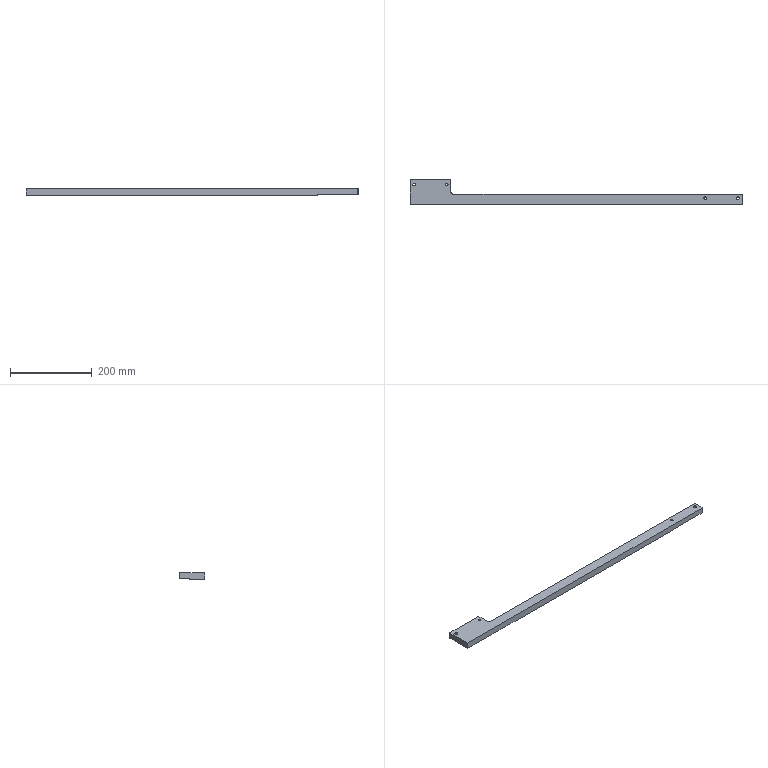Part | NX | features BREP 1 | 1 solid | 26 faces | box 812 x 62 x 16 mm | volume 388249 mm3 | plane 17 | cylinder 9 | commonest cylinder face diameters 6.5 x8 10 x1
STEP:
#1=CARTESIAN_POINT('',(798.75,16.,1.));
#2=VERTEX_POINT('',#1);
#3=CARTESIAN_POINT('',(805.25,16.,1.));
#4=VERTEX_POINT('',#3);
#5=CARTESIAN_POINT('',(802.,16.,1.));
#6=DIRECTION('',(0.,0.,1.));
#7=DIRECTION('',(1.,0.,0.));
#8=AXIS2_PLACEMENT_3D('',#5,#6,#7);
#9=CIRCLE('',#8,3.25);
#10=EDGE_CURVE('',#2,#4,#9,.T.);
#11=ORIENTED_EDGE('',*,*,#10,.F.);
#12=CARTESIAN_POINT('',(798.75,16.,16.));
#13=VERTEX_POINT('',#12);
#14=CARTESIAN_POINT('',(798.75,16.,16.));
#15=DIRECTION('',(0.,0.,1.));
#16=VECTOR('',#15,1000.);
#17=LINE('',#14,#16);
#18=EDGE_CURVE('',#13,#2,#17,.F.);
#19=ORIENTED_EDGE('',*,*,#18,.F.);
#20=CARTESIAN_POINT('',(805.25,16.,16.));
#21=VERTEX_POINT('',#20);
#22=CARTESIAN_POINT('',(802.,16.,16.));
#23=DIRECTION('',(0.,0.,1.));
#24=DIRECTION('',(1.,0.,0.));
#25=AXIS2_PLACEMENT_3D('',#22,#23,#24);
#26=CIRCLE('',#25,3.25);
#27=EDGE_CURVE('',#13,#21,#26,.T.);
#28=ORIENTED_EDGE('',*,*,#27,.T.);
#29=CARTESIAN_POINT('',(805.25,16.,16.));
#30=DIRECTION('',(0.,0.,1.));
#31=VECTOR('',#30,1000.);
#32=LINE('',#29,#31);
#33=EDGE_CURVE('',#21,#4,#32,.F.);
#34=ORIENTED_EDGE('',*,*,#33,.T.);
#35=EDGE_LOOP('',(#11,#19,#28,#34));
#36=FACE_BOUND('',#35,.T.);
#37=CARTESIAN_POINT('',(802.,16.,16.));
#38=DIRECTION('',(0.,0.,1.));
#39=DIRECTION('',(1.,0.,0.));
#40=AXIS2_PLACEMENT_3D('',#37,#38,#39);
#41=CYLINDRICAL_SURFACE('',#40,3.25);
#42=ADVANCED_FACE('',(#36),#41,.F.);
#43=CARTESIAN_POINT('',(718.75,16.,1.));
#44=VERTEX_POINT('',#43);
#45=CARTESIAN_POINT('',(725.25,16.,1.));
#46=VERTEX_POINT('',#45);
#47=CARTESIAN_POINT('',(722.,16.,1.));
#48=DIRECTION('',(0.,0.,1.));
#49=DIRECTION('',(1.,0.,0.));
#50=AXIS2_PLACEMENT_3D('',#47,#48,#49);
#51=CIRCLE('',#50,3.25);
#52=EDGE_CURVE('',#44,#46,#51,.T.);
#53=ORIENTED_EDGE('',*,*,#52,.F.);
#54=CARTESIAN_POINT('',(718.75,16.,16.));
#55=VERTEX_POINT('',#54);
#56=CARTESIAN_POINT('',(718.75,16.,16.));
#57=DIRECTION('',(0.,0.,1.));
#58=VECTOR('',#57,1000.);
#59=LINE('',#56,#58);
#60=EDGE_CURVE('',#55,#44,#59,.F.);
#61=ORIENTED_EDGE('',*,*,#60,.F.);
#62=CARTESIAN_POINT('',(725.25,16.,16.));
#63=VERTEX_POINT('',#62);
#64=CARTESIAN_POINT('',(722.,16.,16.));
#65=DIRECTION('',(0.,0.,1.));
#66=DIRECTION('',(1.,0.,0.));
#67=AXIS2_PLACEMENT_3D('',#64,#65,#66);
#68=CIRCLE('',#67,3.25);
#69=EDGE_CURVE('',#55,#63,#68,.T.);
#70=ORIENTED_EDGE('',*,*,#69,.T.);
#71=CARTESIAN_POINT('',(725.25,16.,16.));
#72=DIRECTION('',(0.,0.,1.));
#73=VECTOR('',#72,1000.);
#74=LINE('',#71,#73);
#75=EDGE_CURVE('',#63,#46,#74,.F.);
#76=ORIENTED_EDGE('',*,*,#75,.T.);
#77=EDGE_LOOP('',(#53,#61,#70,#76));
#78=FACE_BOUND('',#77,.T.);
#79=CARTESIAN_POINT('',(722.,16.,16.));
#80=DIRECTION('',(0.,0.,1.));
#81=DIRECTION('',(1.,0.,0.));
#82=AXIS2_PLACEMENT_3D('',#79,#80,#81);
#83=CYLINDRICAL_SURFACE('',#82,3.25);
#84=ADVANCED_FACE('',(#78),#83,.F.);
#85=CARTESIAN_POINT('',(6.75,49.,1.));
#86=VERTEX_POINT('',#85);
#87=CARTESIAN_POINT('',(13.25,49.,1.));
#88=VERTEX_POINT('',#87);
#89=CARTESIAN_POINT('',(10.,49.,1.));
#90=DIRECTION('',(0.,0.,1.));
#91=DIRECTION('',(1.,0.,0.));
#92=AXIS2_PLACEMENT_3D('',#89,#90,#91);
#93=CIRCLE('',#92,3.25);
#94=EDGE_CURVE('',#86,#88,#93,.T.);
#95=ORIENTED_EDGE('',*,*,#94,.F.);
#96=CARTESIAN_POINT('',(6.75,49.,16.));
#97=VERTEX_POINT('',#96);
#98=CARTESIAN_POINT('',(6.75,49.,16.));
#99=DIRECTION('',(0.,0.,1.));
#100=VECTOR('',#99,1000.);
#101=LINE('',#98,#100);
#102=EDGE_CURVE('',#97,#86,#101,.F.);
#103=ORIENTED_EDGE('',*,*,#102,.F.);
#104=CARTESIAN_POINT('',(13.25,49.,16.));
#105=VERTEX_POINT('',#104);
#106=CARTESIAN_POINT('',(10.,49.,16.));
#107=DIRECTION('',(0.,0.,1.));
#108=DIRECTION('',(1.,0.,0.));
#109=AXIS2_PLACEMENT_3D('',#106,#107,#108);
#110=CIRCLE('',#109,3.25);
#111=EDGE_CURVE('',#97,#105,#110,.T.);
#112=ORIENTED_EDGE('',*,*,#111,.T.);
#113=CARTESIAN_POINT('',(13.25,49.,16.));
#114=DIRECTION('',(0.,0.,1.));
#115=VECTOR('',#114,1000.);
#116=LINE('',#113,#115);
#117=EDGE_CURVE('',#105,#88,#116,.F.);
#118=ORIENTED_EDGE('',*,*,#117,.T.);
#119=EDGE_LOOP('',(#95,#103,#112,#118));
#120=FACE_BOUND('',#119,.T.);
#121=CARTESIAN_POINT('',(10.,49.,16.));
#122=DIRECTION('',(0.,0.,1.));
#123=DIRECTION('',(1.,0.,0.));
#124=AXIS2_PLACEMENT_3D('',#121,#122,#123);
#125=CYLINDRICAL_SURFACE('',#124,3.25);
#126=ADVANCED_FACE('',(#120),#125,.F.);
#127=CARTESIAN_POINT('',(86.75,49.,1.));
#128=VERTEX_POINT('',#127);
#129=CARTESIAN_POINT('',(93.25,49.,1.));
#130=VERTEX_POINT('',#129);
#131=CARTESIAN_POINT('',(90.,49.,1.));
#132=DIRECTION('',(0.,0.,1.));
#133=DIRECTION('',(1.,0.,0.));
#134=AXIS2_PLACEMENT_3D('',#131,#132,#133);
#135=CIRCLE('',#134,3.25);
#136=EDGE_CURVE('',#128,#130,#135,.T.);
#137=ORIENTED_EDGE('',*,*,#136,.F.);
#138=CARTESIAN_POINT('',(86.75,49.,16.));
#139=VERTEX_POINT('',#138);
#140=CARTESIAN_POINT('',(86.75,49.,16.));
#141=DIRECTION('',(0.,0.,1.));
#142=VECTOR('',#141,1000.);
#143=LINE('',#140,#142);
#144=EDGE_CURVE('',#139,#128,#143,.F.);
#145=ORIENTED_EDGE('',*,*,#144,.F.);
#146=CARTESIAN_POINT('',(93.25,49.,16.));
#147=VERTEX_POINT('',#146);
#148=CARTESIAN_POINT('',(90.,49.,16.));
#149=DIRECTION('',(0.,0.,1.));
#150=DIRECTION('',(1.,0.,0.));
#151=AXIS2_PLACEMENT_3D('',#148,#149,#150);
#152=CIRCLE('',#151,3.25);
#153=EDGE_CURVE('',#139,#147,#152,.T.);
#154=ORIENTED_EDGE('',*,*,#153,.T.);
#155=CARTESIAN_POINT('',(93.25,49.,16.));
#156=DIRECTION('',(0.,0.,1.));
#157=VECTOR('',#156,1000.);
#158=LINE('',#155,#157);
#159=EDGE_CURVE('',#147,#130,#158,.F.);
#160=ORIENTED_EDGE('',*,*,#159,.T.);
#161=EDGE_LOOP('',(#137,#145,#154,#160));
#162=FACE_BOUND('',#161,.T.);
#163=CARTESIAN_POINT('',(90.,49.,16.));
#164=DIRECTION('',(0.,0.,1.));
#165=DIRECTION('',(1.,0.,0.));
#166=AXIS2_PLACEMENT_3D('',#163,#164,#165);
#167=CYLINDRICAL_SURFACE('',#166,3.25);
#168=ADVANCED_FACE('',(#162),#167,.F.);
#169=CARTESIAN_POINT('',(1.,62.,1.));
#170=VERTEX_POINT('',#169);
#171=CARTESIAN_POINT('',(99.,62.,1.));
#172=VERTEX_POINT('',#171);
#173=CARTESIAN_POINT('',(0.,62.,1.));
#174=DIRECTION('',(1.,0.,0.));
#175=VECTOR('',#174,1000.);
#176=LINE('',#173,#175);
#177=EDGE_CURVE('',#170,#172,#176,.T.);
#178=ORIENTED_EDGE('',*,*,#177,.F.);
#179=CARTESIAN_POINT('',(1.,62.,16.));
#180=VERTEX_POINT('',#179);
#181=CARTESIAN_POINT('',(1.,62.,16.));
#182=DIRECTION('',(0.,0.,1.));
#183=VECTOR('',#182,1000.);
#184=LINE('',#181,#183);
#185=EDGE_CURVE('',#170,#180,#184,.T.);
#186=ORIENTED_EDGE('',*,*,#185,.T.);
#187=CARTESIAN_POINT('',(99.,62.,16.));
#188=VERTEX_POINT('',#187);
#189=CARTESIAN_POINT('',(100.,62.,16.));
#190=DIRECTION('',(-1.,0.,0.));
#191=VECTOR('',#190,1000.);
#192=LINE('',#189,#191);
#193=EDGE_CURVE('',#188,#180,#192,.T.);
#194=ORIENTED_EDGE('',*,*,#193,.F.);
#195=CARTESIAN_POINT('',(99.,62.,16.));
#196=DIRECTION('',(0.,0.,-1.));
#197=VECTOR('',#196,1000.);
#198=LINE('',#195,#197);
#199=EDGE_CURVE('',#188,#172,#198,.T.);
#200=ORIENTED_EDGE('',*,*,#199,.T.);
#201=EDGE_LOOP('',(#178,#186,#194,#200));
#202=FACE_BOUND('',#201,.T.);
#203=CARTESIAN_POINT('',(100.,62.,16.));
#204=DIRECTION('',(0.,-1.,0.));
#205=DIRECTION('',(0.,0.,-1.));
#206=AXIS2_PLACEMENT_3D('',#203,#204,#205);
#207=PLANE('',#206);
#208=ADVANCED_FACE('',(#202),#207,.F.);
#209=CARTESIAN_POINT('',(100.,61.,1.));
#210=VERTEX_POINT('',#209);
#211=CARTESIAN_POINT('',(100.,61.,16.));
#212=VERTEX_POINT('',#211);
#213=CARTESIAN_POINT('',(100.,61.,16.));
#214=DIRECTION('',(0.,0.,1.));
#215=VECTOR('',#214,1000.);
#216=LINE('',#213,#215);
#217=EDGE_CURVE('',#210,#212,#216,.T.);
#218=ORIENTED_EDGE('',*,*,#217,.F.);
#219=CARTESIAN_POINT('',(99.,62.,1.));
#220=DIRECTION('',(-0.7071,0.7071,0.));
#221=VECTOR('',#220,1000.);
#222=LINE('',#219,#221);
#223=EDGE_CURVE('',#210,#172,#222,.T.);
#224=ORIENTED_EDGE('',*,*,#223,.T.);
#225=ORIENTED_EDGE('',*,*,#199,.F.);
#226=CARTESIAN_POINT('',(80.5,80.5,16.));
#227=DIRECTION('',(-0.7071,0.7071,0.));
#228=VECTOR('',#227,1000.);
#229=LINE('',#226,#228);
#230=EDGE_CURVE('',#212,#188,#229,.T.);
#231=ORIENTED_EDGE('',*,*,#230,.F.);
#232=EDGE_LOOP('',(#218,#224,#225,#231));
#233=FACE_BOUND('',#232,.T.);
#234=CARTESIAN_POINT('',(99.,62.,16.));
#235=DIRECTION('',(-0.7071,-0.7071,0.));
#236=DIRECTION('',(-0.7071,0.7071,0.));
#237=AXIS2_PLACEMENT_3D('',#234,#235,#236);
#238=PLANE('',#237);
#239=ADVANCED_FACE('',(#233),#238,.F.);
#240=ORIENTED_EDGE('',*,*,#185,.F.);
#241=CARTESIAN_POINT('',(0.,61.,1.));
#242=VERTEX_POINT('',#241);
#243=CARTESIAN_POINT('',(0.,61.,1.));
#244=DIRECTION('',(-0.7071,-0.7071,0.));
#245=VECTOR('',#244,1000.);
#246=LINE('',#243,#245);
#247=EDGE_CURVE('',#170,#242,#246,.T.);
#248=ORIENTED_EDGE('',*,*,#247,.T.);
#249=CARTESIAN_POINT('',(0.,61.,16.));
#250=VERTEX_POINT('',#249);
#251=CARTESIAN_POINT('',(0.,61.,16.));
#252=DIRECTION('',(0.,0.,-1.));
#253=VECTOR('',#252,1000.);
#254=LINE('',#251,#253);
#255=EDGE_CURVE('',#250,#242,#254,.T.);
#256=ORIENTED_EDGE('',*,*,#255,.F.);
#257=CARTESIAN_POINT('',(-30.5,30.5,16.));
#258=DIRECTION('',(-0.7071,-0.7071,0.));
#259=VECTOR('',#258,1000.);
#260=LINE('',#257,#259);
#261=EDGE_CURVE('',#180,#250,#260,.T.);
#262=ORIENTED_EDGE('',*,*,#261,.F.);
#263=EDGE_LOOP('',(#240,#248,#256,#262));
#264=FACE_BOUND('',#263,.T.);
#265=CARTESIAN_POINT('',(0.,61.,16.));
#266=DIRECTION('',(0.7071,-0.7071,0.));
#267=DIRECTION('',(0.,0.,-1.));
#268=AXIS2_PLACEMENT_3D('',#265,#266,#267);
#269=PLANE('',#268);
#270=ADVANCED_FACE('',(#264),#269,.F.);
#271=CARTESIAN_POINT('',(0.,36.,1.));
#272=VERTEX_POINT('',#271);
#273=CARTESIAN_POINT('',(0.,36.,1.));
#274=DIRECTION('',(0.,1.,0.));
#275=VECTOR('',#274,1000.);
#276=LINE('',#273,#275);
#277=EDGE_CURVE('',#272,#242,#276,.T.);
#278=ORIENTED_EDGE('',*,*,#277,.F.);
#279=CARTESIAN_POINT('',(0.,36.,0.));
#280=VERTEX_POINT('',#279);
#281=CARTESIAN_POINT('',(0.,36.,1.));
#282=DIRECTION('',(0.,0.,-1.));
#283=VECTOR('',#282,1000.);
#284=LINE('',#281,#283);
#285=EDGE_CURVE('',#272,#280,#284,.T.);
#286=ORIENTED_EDGE('',*,*,#285,.T.);
#287=CARTESIAN_POINT('',(0.,1.,0.));
#288=VERTEX_POINT('',#287);
#289=CARTESIAN_POINT('',(0.,62.,0.));
#290=DIRECTION('',(0.,-1.,0.));
#291=VECTOR('',#290,1000.);
#292=LINE('',#289,#291);
#293=EDGE_CURVE('',#280,#288,#292,.T.);
#294=ORIENTED_EDGE('',*,*,#293,.T.);
#295=CARTESIAN_POINT('',(0.,1.,16.));
#296=VERTEX_POINT('',#295);
#297=CARTESIAN_POINT('',(0.,1.,16.));
#298=DIRECTION('',(0.,0.,1.));
#299=VECTOR('',#298,1000.);
#300=LINE('',#297,#299);
#301=EDGE_CURVE('',#288,#296,#300,.T.);
#302=ORIENTED_EDGE('',*,*,#301,.T.);
#303=CARTESIAN_POINT('',(0.,62.,16.));
#304=DIRECTION('',(0.,-1.,0.));
#305=VECTOR('',#304,1000.);
#306=LINE('',#303,#305);
#307=EDGE_CURVE('',#250,#296,#306,.T.);
#308=ORIENTED_EDGE('',*,*,#307,.F.);
#309=ORIENTED_EDGE('',*,*,#255,.T.);
#310=EDGE_LOOP('',(#278,#286,#294,#302,#308,#309));
#311=FACE_BOUND('',#310,.T.);
#312=CARTESIAN_POINT('',(0.,62.,16.));
#313=DIRECTION('',(1.,0.,0.));
#314=DIRECTION('',(0.,1.,0.));
#315=AXIS2_PLACEMENT_3D('',#312,#313,#314);
#316=PLANE('',#315);
#317=ADVANCED_FACE('',(#311),#316,.F.);
#318=CARTESIAN_POINT('',(1.,0.,0.));
#319=VERTEX_POINT('',#318);
#320=CARTESIAN_POINT('',(712.,0.,0.));
#321=VERTEX_POINT('',#320);
#322=CARTESIAN_POINT('',(0.,0.,0.));
#323=DIRECTION('',(1.,0.,0.));
#324=VECTOR('',#323,1000.);
#325=LINE('',#322,#324);
#326=EDGE_CURVE('',#319,#321,#325,.T.);
#327=ORIENTED_EDGE('',*,*,#326,.T.);
#328=CARTESIAN_POINT('',(712.,0.,1.));
#329=VERTEX_POINT('',#328);
#330=CARTESIAN_POINT('',(712.,0.,16.));
#331=DIRECTION('',(0.,0.,1.));
#332=VECTOR('',#331,1000.);
#333=LINE('',#330,#332);
#334=EDGE_CURVE('',#321,#329,#333,.T.);
#335=ORIENTED_EDGE('',*,*,#334,.T.);
#336=CARTESIAN_POINT('',(811.,0.,1.));
#337=VERTEX_POINT('',#336);
#338=CARTESIAN_POINT('',(0.,0.,1.));
#339=DIRECTION('',(1.,0.,0.));
#340=VECTOR('',#339,1000.);
#341=LINE('',#338,#340);
#342=EDGE_CURVE('',#329,#337,#341,.T.);
#343=ORIENTED_EDGE('',*,*,#342,.T.);
#344=CARTESIAN_POINT('',(811.,0.,16.));
#345=VERTEX_POINT('',#344);
#346=CARTESIAN_POINT('',(811.,0.,16.));
#347=DIRECTION('',(0.,0.,1.));
#348=VECTOR('',#347,1000.);
#349=LINE('',#346,#348);
#350=EDGE_CURVE('',#337,#345,#349,.T.);
#351=ORIENTED_EDGE('',*,*,#350,.T.);
#352=CARTESIAN_POINT('',(1.,0.,16.));
#353=VERTEX_POINT('',#352);
#354=CARTESIAN_POINT('',(0.,0.,16.));
#355=DIRECTION('',(1.,0.,0.));
#356=VECTOR('',#355,1000.);
#357=LINE('',#354,#356);
#358=EDGE_CURVE('',#353,#345,#357,.T.);
#359=ORIENTED_EDGE('',*,*,#358,.F.);
#360=CARTESIAN_POINT('',(1.,0.,16.));
#361=DIRECTION('',(0.,0.,-1.));
#362=VECTOR('',#361,1000.);
#363=LINE('',#360,#362);
#364=EDGE_CURVE('',#353,#319,#363,.T.);
#365=ORIENTED_EDGE('',*,*,#364,.T.);
#366=EDGE_LOOP('',(#327,#335,#343,#351,#359,#365));
#367=FACE_BOUND('',#366,.T.);
#368=CARTESIAN_POINT('',(0.,0.,16.));
#369=DIRECTION('',(0.,1.,0.));
#370=DIRECTION('',(1.,0.,0.));
#371=AXIS2_PLACEMENT_3D('',#368,#369,#370);
#372=PLANE('',#371);
#373=ADVANCED_FACE('',(#367),#372,.F.);
#374=CARTESIAN_POINT('',(812.,1.,16.));
#375=VERTEX_POINT('',#374);
#376=CARTESIAN_POINT('',(812.,1.,1.));
#377=VERTEX_POINT('',#376);
#378=CARTESIAN_POINT('',(812.,1.,16.));
#379=DIRECTION('',(0.,0.,-1.));
#380=VECTOR('',#379,1000.);
#381=LINE('',#378,#380);
#382=EDGE_CURVE('',#375,#377,#381,.T.);
#383=ORIENTED_EDGE('',*,*,#382,.T.);
#384=CARTESIAN_POINT('',(812.,25.,1.));
#385=VERTEX_POINT('',#384);
#386=CARTESIAN_POINT('',(812.,26.,1.));
#387=DIRECTION('',(0.,-1.,0.));
#388=VECTOR('',#387,1000.);
#389=LINE('',#386,#388);
#390=EDGE_CURVE('',#385,#377,#389,.T.);
#391=ORIENTED_EDGE('',*,*,#390,.F.);
#392=CARTESIAN_POINT('',(812.,25.,16.));
#393=VERTEX_POINT('',#392);
#394=CARTESIAN_POINT('',(812.,25.,16.));
#395=DIRECTION('',(0.,0.,1.));
#396=VECTOR('',#395,1000.);
#397=LINE('',#394,#396);
#398=EDGE_CURVE('',#385,#393,#397,.T.);
#399=ORIENTED_EDGE('',*,*,#398,.T.);
#400=CARTESIAN_POINT('',(812.,0.,16.));
#401=DIRECTION('',(0.,1.,0.));
#402=VECTOR('',#401,1000.);
#403=LINE('',#400,#402);
#404=EDGE_CURVE('',#375,#393,#403,.T.);
#405=ORIENTED_EDGE('',*,*,#404,.F.);
#406=EDGE_LOOP('',(#383,#391,#399,#405));
#407=FACE_BOUND('',#406,.T.);
#408=CARTESIAN_POINT('',(812.,0.,16.));
#409=DIRECTION('',(-1.,0.,0.));
#410=DIRECTION('',(0.,0.,1.));
#411=AXIS2_PLACEMENT_3D('',#408,#409,#410);
#412=PLANE('',#411);
#413=ADVANCED_FACE('',(#407),#412,.F.);
#414=CARTESIAN_POINT('',(712.,26.,1.));
#415=VERTEX_POINT('',#414);
#416=CARTESIAN_POINT('',(811.,26.,1.));
#417=VERTEX_POINT('',#416);
#418=CARTESIAN_POINT('',(712.,26.,1.));
#419=DIRECTION('',(1.,0.,0.));
#420=VECTOR('',#419,1000.);
#421=LINE('',#418,#420);
#422=EDGE_CURVE('',#415,#417,#421,.T.);
#423=ORIENTED_EDGE('',*,*,#422,.F.);
#424=CARTESIAN_POINT('',(712.,26.,0.));
#425=VERTEX_POINT('',#424);
#426=CARTESIAN_POINT('',(712.,26.,1.));
#427=DIRECTION('',(0.,0.,-1.));
#428=VECTOR('',#427,1000.);
#429=LINE('',#426,#428);
#430=EDGE_CURVE('',#415,#425,#429,.T.);
#431=ORIENTED_EDGE('',*,*,#430,.T.);
#432=CARTESIAN_POINT('',(105.,26.,0.));
#433=VERTEX_POINT('',#432);
#434=CARTESIAN_POINT('',(812.,26.,0.));
#435=DIRECTION('',(-1.,0.,0.));
#436=VECTOR('',#435,1000.);
#437=LINE('',#434,#436);
#438=EDGE_CURVE('',#425,#433,#437,.T.);
#439=ORIENTED_EDGE('',*,*,#438,.T.);
#440=CARTESIAN_POINT('',(105.,26.,16.));
#441=VERTEX_POINT('',#440);
#442=CARTESIAN_POINT('',(105.,26.,16.));
#443=DIRECTION('',(0.,0.,1.));
#444=VECTOR('',#443,1000.);
#445=LINE('',#442,#444);
#446=EDGE_CURVE('',#433,#441,#445,.T.);
#447=ORIENTED_EDGE('',*,*,#446,.T.);
#448=CARTESIAN_POINT('',(811.,26.,16.));
#449=VERTEX_POINT('',#448);
#450=CARTESIAN_POINT('',(812.,26.,16.));
#451=DIRECTION('',(-1.,0.,0.));
#452=VECTOR('',#451,1000.);
#453=LINE('',#450,#452);
#454=EDGE_CURVE('',#449,#441,#453,.T.);
#455=ORIENTED_EDGE('',*,*,#454,.F.);
#456=CARTESIAN_POINT('',(811.,26.,16.));
#457=DIRECTION('',(0.,0.,-1.));
#458=VECTOR('',#457,1000.);
#459=LINE('',#456,#458);
#460=EDGE_CURVE('',#449,#417,#459,.T.);
#461=ORIENTED_EDGE('',*,*,#460,.T.);
#462=EDGE_LOOP('',(#423,#431,#439,#447,#455,#461));
#463=FACE_BOUND('',#462,.T.);
#464=CARTESIAN_POINT('',(812.,26.,16.));
#465=DIRECTION('',(0.,-1.,0.));
#466=DIRECTION('',(0.,0.,-1.));
#467=AXIS2_PLACEMENT_3D('',#464,#465,#466);
#468=PLANE('',#467);
#469=ADVANCED_FACE('',(#463),#468,.F.);
#470=CARTESIAN_POINT('',(100.,31.,0.));
#471=VERTEX_POINT('',#470);
#472=CARTESIAN_POINT('',(100.,36.,0.));
#473=VERTEX_POINT('',#472);
#474=CARTESIAN_POINT('',(100.,26.,0.));
#475=DIRECTION('',(0.,1.,0.));
#476=VECTOR('',#475,1000.);
#477=LINE('',#474,#476);
#478=EDGE_CURVE('',#471,#473,#477,.T.);
#479=ORIENTED_EDGE('',*,*,#478,.T.);
#480=CARTESIAN_POINT('',(100.,36.,1.));
#481=VERTEX_POINT('',#480);
#482=CARTESIAN_POINT('',(100.,36.,1.));
#483=DIRECTION('',(0.,0.,-1.));
#484=VECTOR('',#483,1000.);
#485=LINE('',#482,#484);
#486=EDGE_CURVE('',#481,#473,#485,.T.);
#487=ORIENTED_EDGE('',*,*,#486,.F.);
#488=CARTESIAN_POINT('',(100.,36.,1.));
#489=DIRECTION('',(0.,-1.,0.));
#490=VECTOR('',#489,1000.);
#491=LINE('',#488,#490);
#492=EDGE_CURVE('',#210,#481,#491,.T.);
#493=ORIENTED_EDGE('',*,*,#492,.F.);
#494=ORIENTED_EDGE('',*,*,#217,.T.);
#495=CARTESIAN_POINT('',(100.,31.,16.));
#496=VERTEX_POINT('',#495);
#497=CARTESIAN_POINT('',(100.,26.,16.));
#498=DIRECTION('',(0.,1.,0.));
#499=VECTOR('',#498,1000.);
#500=LINE('',#497,#499);
#501=EDGE_CURVE('',#496,#212,#500,.T.);
#502=ORIENTED_EDGE('',*,*,#501,.F.);
#503=CARTESIAN_POINT('',(100.,31.,0.));
#504=DIRECTION('',(0.,0.,-1.));
#505=VECTOR('',#504,1000.);
#506=LINE('',#503,#505);
#507=EDGE_CURVE('',#496,#471,#506,.T.);
#508=ORIENTED_EDGE('',*,*,#507,.T.);
#509=EDGE_LOOP('',(#479,#487,#493,#494,#502,#508));
#510=FACE_BOUND('',#509,.T.);
#511=CARTESIAN_POINT('',(100.,26.,16.));
#512=DIRECTION('',(-1.,0.,0.));
#513=DIRECTION('',(0.,0.,1.));
#514=AXIS2_PLACEMENT_3D('',#511,#512,#513);
#515=PLANE('',#514);
#516=ADVANCED_FACE('',(#510),#515,.F.);
#517=ORIENTED_EDGE('',*,*,#358,.T.);
#518=CARTESIAN_POINT('',(405.5,-405.5,16.));
#519=DIRECTION('',(0.7071,0.7071,0.));
#520=VECTOR('',#519,1000.);
#521=LINE('',#518,#520);
#522=EDGE_CURVE('',#345,#375,#521,.T.);
#523=ORIENTED_EDGE('',*,*,#522,.T.);
#524=ORIENTED_EDGE('',*,*,#404,.T.);
#525=CARTESIAN_POINT('',(418.5,418.5,16.));
#526=DIRECTION('',(-0.7071,0.7071,0.));
#527=VECTOR('',#526,1000.);
#528=LINE('',#525,#527);
#529=EDGE_CURVE('',#393,#449,#528,.T.);
#530=ORIENTED_EDGE('',*,*,#529,.T.);
#531=ORIENTED_EDGE('',*,*,#454,.T.);
#532=CARTESIAN_POINT('',(105.,31.,16.));
#533=DIRECTION('',(0.,0.,-1.));
#534=DIRECTION('',(1.,0.,0.));
#535=AXIS2_PLACEMENT_3D('',#532,#533,#534);
#536=CIRCLE('',#535,5.);
#537=EDGE_CURVE('',#441,#496,#536,.T.);
#538=ORIENTED_EDGE('',*,*,#537,.T.);
#539=ORIENTED_EDGE('',*,*,#501,.T.);
#540=ORIENTED_EDGE('',*,*,#230,.T.);
#541=ORIENTED_EDGE('',*,*,#193,.T.);
#542=ORIENTED_EDGE('',*,*,#261,.T.);
#543=ORIENTED_EDGE('',*,*,#307,.T.);
#544=CARTESIAN_POINT('',(0.5,0.5,16.));
#545=DIRECTION('',(0.7071,-0.7071,0.));
#546=VECTOR('',#545,1000.);
#547=LINE('',#544,#546);
#548=EDGE_CURVE('',#296,#353,#547,.T.);
#549=ORIENTED_EDGE('',*,*,#548,.T.);
#550=EDGE_LOOP('',(#517,#523,#524,#530,#531,#538,#539,#540,#541,#542,#543,#549));
#551=FACE_BOUND('',#550,.T.);
#552=CARTESIAN_POINT('',(802.,16.,16.));
#553=DIRECTION('',(0.,0.,1.));
#554=DIRECTION('',(1.,0.,0.));
#555=AXIS2_PLACEMENT_3D('',#552,#553,#554);
#556=CIRCLE('',#555,3.25);
#557=EDGE_CURVE('',#21,#13,#556,.T.);
#558=ORIENTED_EDGE('',*,*,#557,.F.);
#559=ORIENTED_EDGE('',*,*,#27,.F.);
#560=EDGE_LOOP('',(#558,#559));
#561=FACE_BOUND('',#560,.T.);
#562=CARTESIAN_POINT('',(722.,16.,16.));
#563=DIRECTION('',(0.,0.,1.));
#564=DIRECTION('',(1.,0.,0.));
#565=AXIS2_PLACEMENT_3D('',#562,#563,#564);
#566=CIRCLE('',#565,3.25);
#567=EDGE_CURVE('',#63,#55,#566,.T.);
#568=ORIENTED_EDGE('',*,*,#567,.F.);
#569=ORIENTED_EDGE('',*,*,#69,.F.);
#570=EDGE_LOOP('',(#568,#569));
#571=FACE_BOUND('',#570,.T.);
#572=CARTESIAN_POINT('',(10.,49.,16.));
#573=DIRECTION('',(0.,0.,1.));
#574=DIRECTION('',(1.,0.,0.));
#575=AXIS2_PLACEMENT_3D('',#572,#573,#574);
#576=CIRCLE('',#575,3.25);
#577=EDGE_CURVE('',#105,#97,#576,.T.);
#578=ORIENTED_EDGE('',*,*,#577,.F.);
#579=ORIENTED_EDGE('',*,*,#111,.F.);
#580=EDGE_LOOP('',(#578,#579));
#581=FACE_BOUND('',#580,.T.);
#582=CARTESIAN_POINT('',(90.,49.,16.));
#583=DIRECTION('',(0.,0.,1.));
#584=DIRECTION('',(1.,0.,0.));
#585=AXIS2_PLACEMENT_3D('',#582,#583,#584);
#586=CIRCLE('',#585,3.25);
#587=EDGE_CURVE('',#147,#139,#586,.T.);
#588=ORIENTED_EDGE('',*,*,#587,.F.);
#589=ORIENTED_EDGE('',*,*,#153,.F.);
#590=EDGE_LOOP('',(#588,#589));
#591=FACE_BOUND('',#590,.T.);
#592=CARTESIAN_POINT('',(0.,0.,16.));
#593=DIRECTION('',(0.,0.,1.));
#594=DIRECTION('',(1.,0.,0.));
#595=AXIS2_PLACEMENT_3D('',#592,#593,#594);
#596=PLANE('',#595);
#597=ADVANCED_FACE('',(#551,#561,#571,#581,#591),#596,.T.);
#598=ORIENTED_EDGE('',*,*,#438,.F.);
#599=CARTESIAN_POINT('',(712.,26.,0.));
#600=DIRECTION('',(0.,1.,0.));
#601=VECTOR('',#600,1000.);
#602=LINE('',#599,#601);
#603=EDGE_CURVE('',#321,#425,#602,.T.);
#604=ORIENTED_EDGE('',*,*,#603,.F.);
#605=ORIENTED_EDGE('',*,*,#326,.F.);
#606=CARTESIAN_POINT('',(1.,0.,0.));
#607=DIRECTION('',(-0.7071,0.7071,0.));
#608=VECTOR('',#607,1000.);
#609=LINE('',#606,#608);
#610=EDGE_CURVE('',#319,#288,#609,.T.);
#611=ORIENTED_EDGE('',*,*,#610,.T.);
#612=ORIENTED_EDGE('',*,*,#293,.F.);
#613=CARTESIAN_POINT('',(0.,36.,0.));
#614=DIRECTION('',(-1.,0.,0.));
#615=VECTOR('',#614,1000.);
#616=LINE('',#613,#615);
#617=EDGE_CURVE('',#473,#280,#616,.T.);
#618=ORIENTED_EDGE('',*,*,#617,.F.);
#619=ORIENTED_EDGE('',*,*,#478,.F.);
#620=CARTESIAN_POINT('',(105.,31.,0.));
#621=DIRECTION('',(0.,0.,1.));
#622=DIRECTION('',(1.,0.,0.));
#623=AXIS2_PLACEMENT_3D('',#620,#621,#622);
#624=CIRCLE('',#623,5.);
#625=EDGE_CURVE('',#471,#433,#624,.T.);
#626=ORIENTED_EDGE('',*,*,#625,.T.);
#627=EDGE_LOOP('',(#598,#604,#605,#611,#612,#618,#619,#626));
#628=FACE_BOUND('',#627,.T.);
#629=CARTESIAN_POINT('',(0.,0.,0.));
#630=DIRECTION('',(0.,0.,1.));
#631=DIRECTION('',(1.,0.,0.));
#632=AXIS2_PLACEMENT_3D('',#629,#630,#631);
#633=PLANE('',#632);
#634=ADVANCED_FACE('',(#628),#633,.F.);
#635=CARTESIAN_POINT('',(812.,1.,1.));
#636=DIRECTION('',(-0.7071,-0.7071,0.));
#637=VECTOR('',#636,1000.);
#638=LINE('',#635,#637);
#639=EDGE_CURVE('',#377,#337,#638,.T.);
#640=ORIENTED_EDGE('',*,*,#639,.F.);
#641=ORIENTED_EDGE('',*,*,#382,.F.);
#642=ORIENTED_EDGE('',*,*,#522,.F.);
#643=ORIENTED_EDGE('',*,*,#350,.F.);
#644=EDGE_LOOP('',(#640,#641,#642,#643));
#645=FACE_BOUND('',#644,.T.);
#646=CARTESIAN_POINT('',(812.,1.,16.));
#647=DIRECTION('',(-0.7071,0.7071,0.));
#648=DIRECTION('',(0.,0.,1.));
#649=AXIS2_PLACEMENT_3D('',#646,#647,#648);
#650=PLANE('',#649);
#651=ADVANCED_FACE('',(#645),#650,.F.);
#652=CARTESIAN_POINT('',(811.,26.,1.));
#653=DIRECTION('',(0.7071,-0.7071,0.));
#654=VECTOR('',#653,1000.);
#655=LINE('',#652,#654);
#656=EDGE_CURVE('',#417,#385,#655,.T.);
#657=ORIENTED_EDGE('',*,*,#656,.F.);
#658=ORIENTED_EDGE('',*,*,#460,.F.);
#659=ORIENTED_EDGE('',*,*,#529,.F.);
#660=ORIENTED_EDGE('',*,*,#398,.F.);
#661=EDGE_LOOP('',(#657,#658,#659,#660));
#662=FACE_BOUND('',#661,.T.);
#663=CARTESIAN_POINT('',(811.,26.,16.));
#664=DIRECTION('',(-0.7071,-0.7071,0.));
#665=DIRECTION('',(-0.7071,0.7071,0.));
#666=AXIS2_PLACEMENT_3D('',#663,#664,#665);
#667=PLANE('',#666);
#668=ADVANCED_FACE('',(#662),#667,.F.);
#669=ORIENTED_EDGE('',*,*,#548,.F.);
#670=ORIENTED_EDGE('',*,*,#301,.F.);
#671=ORIENTED_EDGE('',*,*,#610,.F.);
#672=ORIENTED_EDGE('',*,*,#364,.F.);
#673=EDGE_LOOP('',(#669,#670,#671,#672));
#674=FACE_BOUND('',#673,.T.);
#675=CARTESIAN_POINT('',(1.,0.,16.));
#676=DIRECTION('',(0.7071,0.7071,0.));
#677=DIRECTION('',(0.,0.,-1.));
#678=AXIS2_PLACEMENT_3D('',#675,#676,#677);
#679=PLANE('',#678);
#680=ADVANCED_FACE('',(#674),#679,.F.);
#681=ORIENTED_EDGE('',*,*,#537,.F.);
#682=ORIENTED_EDGE('',*,*,#446,.F.);
#683=ORIENTED_EDGE('',*,*,#625,.F.);
#684=ORIENTED_EDGE('',*,*,#507,.F.);
#685=EDGE_LOOP('',(#681,#682,#683,#684));
#686=FACE_BOUND('',#685,.T.);
#687=CARTESIAN_POINT('',(105.,31.,16.));
#688=DIRECTION('',(0.,0.,1.));
#689=DIRECTION('',(1.,0.,0.));
#690=AXIS2_PLACEMENT_3D('',#687,#688,#689);
#691=CYLINDRICAL_SURFACE('',#690,5.);
#692=ADVANCED_FACE('',(#686),#691,.F.);
#693=ORIENTED_EDGE('',*,*,#617,.T.);
#694=ORIENTED_EDGE('',*,*,#285,.F.);
#695=CARTESIAN_POINT('',(0.,36.,1.));
#696=DIRECTION('',(-1.,0.,0.));
#697=VECTOR('',#696,1000.);
#698=LINE('',#695,#697);
#699=EDGE_CURVE('',#481,#272,#698,.T.);
#700=ORIENTED_EDGE('',*,*,#699,.F.);
#701=ORIENTED_EDGE('',*,*,#486,.T.);
#702=EDGE_LOOP('',(#693,#694,#700,#701));
#703=FACE_BOUND('',#702,.T.);
#704=CARTESIAN_POINT('',(0.,36.,1.));
#705=DIRECTION('',(0.,-1.,0.));
#706=DIRECTION('',(-1.,0.,0.));
#707=AXIS2_PLACEMENT_3D('',#704,#705,#706);
#708=PLANE('',#707);
#709=ADVANCED_FACE('',(#703),#708,.F.);
#710=ORIENTED_EDGE('',*,*,#492,.T.);
#711=ORIENTED_EDGE('',*,*,#699,.T.);
#712=ORIENTED_EDGE('',*,*,#277,.T.);
#713=ORIENTED_EDGE('',*,*,#247,.F.);
#714=ORIENTED_EDGE('',*,*,#177,.T.);
#715=ORIENTED_EDGE('',*,*,#223,.F.);
#716=EDGE_LOOP('',(#710,#711,#712,#713,#714,#715));
#717=FACE_BOUND('',#716,.T.);
#718=CARTESIAN_POINT('',(10.,49.,1.));
#719=DIRECTION('',(0.,0.,1.));
#720=DIRECTION('',(1.,0.,0.));
#721=AXIS2_PLACEMENT_3D('',#718,#719,#720);
#722=CIRCLE('',#721,3.25);
#723=EDGE_CURVE('',#88,#86,#722,.T.);
#724=ORIENTED_EDGE('',*,*,#723,.T.);
#725=ORIENTED_EDGE('',*,*,#94,.T.);
#726=EDGE_LOOP('',(#724,#725));
#727=FACE_BOUND('',#726,.T.);
#728=CARTESIAN_POINT('',(90.,49.,1.));
#729=DIRECTION('',(0.,0.,1.));
#730=DIRECTION('',(1.,0.,0.));
#731=AXIS2_PLACEMENT_3D('',#728,#729,#730);
#732=CIRCLE('',#731,3.25);
#733=EDGE_CURVE('',#130,#128,#732,.T.);
#734=ORIENTED_EDGE('',*,*,#733,.T.);
#735=ORIENTED_EDGE('',*,*,#136,.T.);
#736=EDGE_LOOP('',(#734,#735));
#737=FACE_BOUND('',#736,.T.);
#738=CARTESIAN_POINT('',(0.,0.,1.));
#739=DIRECTION('',(0.,0.,-1.));
#740=DIRECTION('',(0.,-1.,0.));
#741=AXIS2_PLACEMENT_3D('',#738,#739,#740);
#742=PLANE('',#741);
#743=ADVANCED_FACE('',(#717,#727,#737),#742,.T.);
#744=ORIENTED_EDGE('',*,*,#603,.T.);
#745=ORIENTED_EDGE('',*,*,#430,.F.);
#746=CARTESIAN_POINT('',(712.,26.,1.));
#747=DIRECTION('',(0.,1.,0.));
#748=VECTOR('',#747,1000.);
#749=LINE('',#746,#748);
#750=EDGE_CURVE('',#329,#415,#749,.T.);
#751=ORIENTED_EDGE('',*,*,#750,.F.);
#752=ORIENTED_EDGE('',*,*,#334,.F.);
#753=EDGE_LOOP('',(#744,#745,#751,#752));
#754=FACE_BOUND('',#753,.T.);
#755=CARTESIAN_POINT('',(712.,26.,1.));
#756=DIRECTION('',(-1.,0.,0.));
#757=DIRECTION('',(0.,0.,1.));
#758=AXIS2_PLACEMENT_3D('',#755,#756,#757);
#759=PLANE('',#758);
#760=ADVANCED_FACE('',(#754),#759,.F.);
#761=ORIENTED_EDGE('',*,*,#750,.T.);
#762=ORIENTED_EDGE('',*,*,#422,.T.);
#763=ORIENTED_EDGE('',*,*,#656,.T.);
#764=ORIENTED_EDGE('',*,*,#390,.T.);
#765=ORIENTED_EDGE('',*,*,#639,.T.);
#766=ORIENTED_EDGE('',*,*,#342,.F.);
#767=EDGE_LOOP('',(#761,#762,#763,#764,#765,#766));
#768=FACE_BOUND('',#767,.T.);
#769=CARTESIAN_POINT('',(802.,16.,1.));
#770=DIRECTION('',(0.,0.,1.));
#771=DIRECTION('',(1.,0.,0.));
#772=AXIS2_PLACEMENT_3D('',#769,#770,#771);
#773=CIRCLE('',#772,3.25);
#774=EDGE_CURVE('',#4,#2,#773,.T.);
#775=ORIENTED_EDGE('',*,*,#774,.T.);
#776=ORIENTED_EDGE('',*,*,#10,.T.);
#777=EDGE_LOOP('',(#775,#776));
#778=FACE_BOUND('',#777,.T.);
#779=CARTESIAN_POINT('',(722.,16.,1.));
#780=DIRECTION('',(0.,0.,1.));
#781=DIRECTION('',(1.,0.,0.));
#782=AXIS2_PLACEMENT_3D('',#779,#780,#781);
#783=CIRCLE('',#782,3.25);
#784=EDGE_CURVE('',#46,#44,#783,.T.);
#785=ORIENTED_EDGE('',*,*,#784,.T.);
#786=ORIENTED_EDGE('',*,*,#52,.T.);
#787=EDGE_LOOP('',(#785,#786));
#788=FACE_BOUND('',#787,.T.);
#789=CARTESIAN_POINT('',(0.,0.,1.));
#790=DIRECTION('',(0.,0.,1.));
#791=DIRECTION('',(1.,0.,0.));
#792=AXIS2_PLACEMENT_3D('',#789,#790,#791);
#793=PLANE('',#792);
#794=ADVANCED_FACE('',(#768,#778,#788),#793,.F.);
#795=ORIENTED_EDGE('',*,*,#144,.T.);
#796=ORIENTED_EDGE('',*,*,#733,.F.);
#797=ORIENTED_EDGE('',*,*,#159,.F.);
#798=ORIENTED_EDGE('',*,*,#587,.T.);
#799=EDGE_LOOP('',(#795,#796,#797,#798));
#800=FACE_BOUND('',#799,.T.);
#801=CARTESIAN_POINT('',(90.,49.,16.));
#802=DIRECTION('',(0.,0.,1.));
#803=DIRECTION('',(1.,0.,0.));
#804=AXIS2_PLACEMENT_3D('',#801,#802,#803);
#805=CYLINDRICAL_SURFACE('',#804,3.25);
#806=ADVANCED_FACE('',(#800),#805,.F.);
#807=ORIENTED_EDGE('',*,*,#102,.T.);
#808=ORIENTED_EDGE('',*,*,#723,.F.);
#809=ORIENTED_EDGE('',*,*,#117,.F.);
#810=ORIENTED_EDGE('',*,*,#577,.T.);
#811=EDGE_LOOP('',(#807,#808,#809,#810));
#812=FACE_BOUND('',#811,.T.);
#813=CARTESIAN_POINT('',(10.,49.,16.));
#814=DIRECTION('',(0.,0.,1.));
#815=DIRECTION('',(1.,0.,0.));
#816=AXIS2_PLACEMENT_3D('',#813,#814,#815);
#817=CYLINDRICAL_SURFACE('',#816,3.25);
#818=ADVANCED_FACE('',(#812),#817,.F.);
#819=ORIENTED_EDGE('',*,*,#60,.T.);
#820=ORIENTED_EDGE('',*,*,#784,.F.);
#821=ORIENTED_EDGE('',*,*,#75,.F.);
#822=ORIENTED_EDGE('',*,*,#567,.T.);
#823=EDGE_LOOP('',(#819,#820,#821,#822));
#824=FACE_BOUND('',#823,.T.);
#825=CARTESIAN_POINT('',(722.,16.,16.));
#826=DIRECTION('',(0.,0.,1.));
#827=DIRECTION('',(1.,0.,0.));
#828=AXIS2_PLACEMENT_3D('',#825,#826,#827);
#829=CYLINDRICAL_SURFACE('',#828,3.25);
#830=ADVANCED_FACE('',(#824),#829,.F.);
#831=ORIENTED_EDGE('',*,*,#18,.T.);
#832=ORIENTED_EDGE('',*,*,#774,.F.);
#833=ORIENTED_EDGE('',*,*,#33,.F.);
#834=ORIENTED_EDGE('',*,*,#557,.T.);
#835=EDGE_LOOP('',(#831,#832,#833,#834));
#836=FACE_BOUND('',#835,.T.);
#837=CARTESIAN_POINT('',(802.,16.,16.));
#838=DIRECTION('',(0.,0.,1.));
#839=DIRECTION('',(1.,0.,0.));
#840=AXIS2_PLACEMENT_3D('',#837,#838,#839);
#841=CYLINDRICAL_SURFACE('',#840,3.25);
#842=ADVANCED_FACE('',(#836),#841,.F.);
#843=CLOSED_SHELL('',(#42,#84,#126,#168,#208,#239,#270,#317,#373,#413,#469,#516,#597,#634,#651,#668,#680,#692,#709,#743,#760,#794,#806,#818,#830,#842));
#844=MANIFOLD_SOLID_BREP('',#843);
#845=(LENGTH_UNIT()NAMED_UNIT(*)SI_UNIT(.MILLI.,.METRE.));
#846=UNCERTAINTY_MEASURE_WITH_UNIT(LENGTH_MEASURE(0.00001),#845,'','');
#847=(NAMED_UNIT(*)PLANE_ANGLE_UNIT()SI_UNIT($,.RADIAN.));
#848=(NAMED_UNIT(*)SI_UNIT($,.STERADIAN.)SOLID_ANGLE_UNIT());
#849=(GEOMETRIC_REPRESENTATION_CONTEXT(3)GLOBAL_UNCERTAINTY_ASSIGNED_CONTEXT((#846))GLOBAL_UNIT_ASSIGNED_CONTEXT((#845,#847,#848))REPRESENTATION_CONTEXT('',''));
#850=ADVANCED_BREP_SHAPE_REPRESENTATION('',(#844),#849);